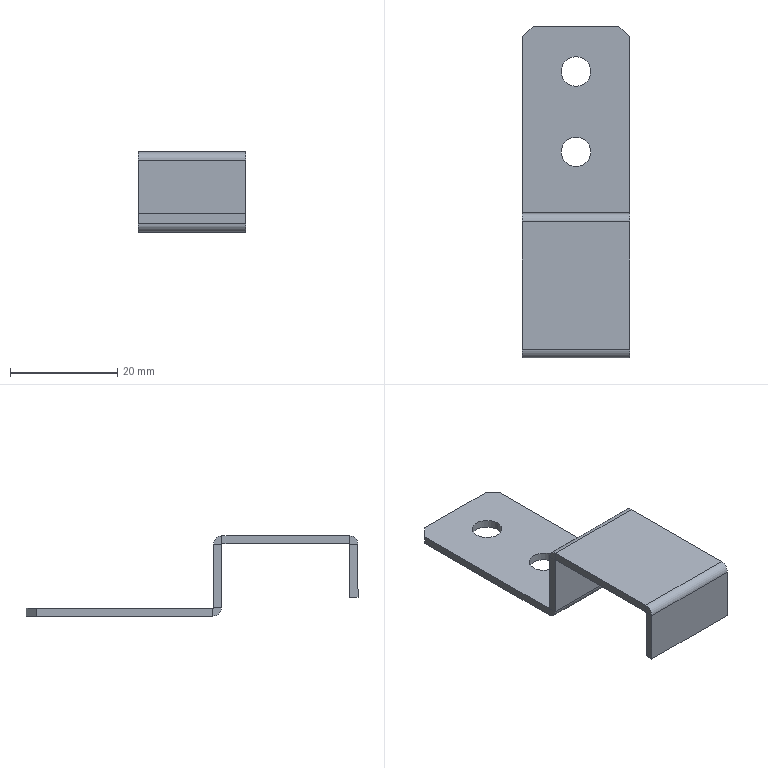Part | SolidWorks | features SplitBody 1 | 1 solid | 36 faces | box 20 x 62 x 15 mm | volume 2455 mm3 | plane 26 | cylinder 10 | commonest cylinder face diameters 5.5 x4 0.2 x3 3.2 x3
STEP:
#1=CARTESIAN_POINT('',(-247.25,40.,-280.));
#2=VERTEX_POINT('',#1);
#3=CARTESIAN_POINT('',(-252.75,40.,-280.));
#4=VERTEX_POINT('',#3);
#5=CARTESIAN_POINT('',(-250.,40.,-280.));
#6=DIRECTION('',(0.,0.,-1.));
#7=DIRECTION('',(-1.,0.,0.));
#8=AXIS2_PLACEMENT_3D('',#5,#6,#7);
#9=CIRCLE('',#8,2.75);
#10=EDGE_CURVE('',#2,#4,#9,.T.);
#11=ORIENTED_EDGE('',*,*,#10,.F.);
#12=CARTESIAN_POINT('',(-247.25,40.,-281.5));
#13=VERTEX_POINT('',#12);
#14=CARTESIAN_POINT('',(-247.25,40.,-221.5));
#15=DIRECTION('',(0.,0.,-1.));
#16=VECTOR('',#15,1000.);
#17=LINE('',#14,#16);
#18=EDGE_CURVE('',#2,#13,#17,.T.);
#19=ORIENTED_EDGE('',*,*,#18,.T.);
#20=CARTESIAN_POINT('',(-252.75,40.,-281.5));
#21=VERTEX_POINT('',#20);
#22=CARTESIAN_POINT('',(-250.,40.,-281.5));
#23=DIRECTION('',(0.,0.,-1.));
#24=DIRECTION('',(-1.,0.,0.));
#25=AXIS2_PLACEMENT_3D('',#22,#23,#24);
#26=CIRCLE('',#25,2.75);
#27=EDGE_CURVE('',#13,#21,#26,.T.);
#28=ORIENTED_EDGE('',*,*,#27,.T.);
#29=CARTESIAN_POINT('',(-252.75,40.,-221.5));
#30=DIRECTION('',(0.,0.,-1.));
#31=VECTOR('',#30,1000.);
#32=LINE('',#29,#31);
#33=EDGE_CURVE('',#4,#21,#32,.T.);
#34=ORIENTED_EDGE('',*,*,#33,.F.);
#35=EDGE_LOOP('',(#11,#19,#28,#34));
#36=FACE_OUTER_BOUND('',#35,.T.);
#37=CARTESIAN_POINT('',(-250.,40.,-221.5));
#38=DIRECTION('',(0.,0.,-1.));
#39=DIRECTION('',(-1.,0.,0.));
#40=AXIS2_PLACEMENT_3D('',#37,#38,#39);
#41=CYLINDRICAL_SURFACE('',#40,2.75);
#42=ADVANCED_FACE('',(#36),#41,.F.);
#43=CARTESIAN_POINT('',(-247.25,55.,-280.));
#44=VERTEX_POINT('',#43);
#45=CARTESIAN_POINT('',(-252.75,55.,-280.));
#46=VERTEX_POINT('',#45);
#47=CARTESIAN_POINT('',(-250.,55.,-280.));
#48=DIRECTION('',(0.,0.,-1.));
#49=DIRECTION('',(-1.,0.,0.));
#50=AXIS2_PLACEMENT_3D('',#47,#48,#49);
#51=CIRCLE('',#50,2.75);
#52=EDGE_CURVE('',#44,#46,#51,.T.);
#53=ORIENTED_EDGE('',*,*,#52,.F.);
#54=CARTESIAN_POINT('',(-247.25,55.,-281.5));
#55=VERTEX_POINT('',#54);
#56=CARTESIAN_POINT('',(-247.25,55.,-221.5));
#57=DIRECTION('',(0.,0.,-1.));
#58=VECTOR('',#57,1000.);
#59=LINE('',#56,#58);
#60=EDGE_CURVE('',#44,#55,#59,.T.);
#61=ORIENTED_EDGE('',*,*,#60,.T.);
#62=CARTESIAN_POINT('',(-252.75,55.,-281.5));
#63=VERTEX_POINT('',#62);
#64=CARTESIAN_POINT('',(-250.,55.,-281.5));
#65=DIRECTION('',(0.,0.,-1.));
#66=DIRECTION('',(-1.,0.,0.));
#67=AXIS2_PLACEMENT_3D('',#64,#65,#66);
#68=CIRCLE('',#67,2.75);
#69=EDGE_CURVE('',#55,#63,#68,.T.);
#70=ORIENTED_EDGE('',*,*,#69,.T.);
#71=CARTESIAN_POINT('',(-252.75,55.,-221.5));
#72=DIRECTION('',(0.,0.,-1.));
#73=VECTOR('',#72,1000.);
#74=LINE('',#71,#73);
#75=EDGE_CURVE('',#46,#63,#74,.T.);
#76=ORIENTED_EDGE('',*,*,#75,.F.);
#77=EDGE_LOOP('',(#53,#61,#70,#76));
#78=FACE_OUTER_BOUND('',#77,.T.);
#79=CARTESIAN_POINT('',(-250.,55.,-221.5));
#80=DIRECTION('',(0.,0.,-1.));
#81=DIRECTION('',(-1.,0.,0.));
#82=AXIS2_PLACEMENT_3D('',#79,#80,#81);
#83=CYLINDRICAL_SURFACE('',#82,2.75);
#84=ADVANCED_FACE('',(#78),#83,.F.);
#85=CARTESIAN_POINT('',(-260.,28.5,-279.9));
#86=VERTEX_POINT('',#85);
#87=CARTESIAN_POINT('',(-260.,27.,-279.9));
#88=VERTEX_POINT('',#87);
#89=CARTESIAN_POINT('',(-260.,28.5,-279.9));
#90=DIRECTION('',(0.,-1.,0.));
#91=VECTOR('',#90,1000.);
#92=LINE('',#89,#91);
#93=EDGE_CURVE('',#86,#88,#92,.T.);
#94=ORIENTED_EDGE('',*,*,#93,.T.);
#95=CARTESIAN_POINT('',(-260.,27.,-268.1));
#96=VERTEX_POINT('',#95);
#97=CARTESIAN_POINT('',(-260.,27.,-268.));
#98=DIRECTION('',(0.,0.,1.));
#99=VECTOR('',#98,1000.);
#100=LINE('',#97,#99);
#101=EDGE_CURVE('',#88,#96,#100,.T.);
#102=ORIENTED_EDGE('',*,*,#101,.T.);
#103=CARTESIAN_POINT('',(-260.,28.5,-268.1));
#104=VERTEX_POINT('',#103);
#105=CARTESIAN_POINT('',(-260.,28.5,-268.1));
#106=DIRECTION('',(0.,1.,0.));
#107=VECTOR('',#106,1000.);
#108=LINE('',#105,#107);
#109=EDGE_CURVE('',#96,#104,#108,.T.);
#110=ORIENTED_EDGE('',*,*,#109,.T.);
#111=CARTESIAN_POINT('',(-260.,28.5,0.));
#112=DIRECTION('',(0.,0.,1.));
#113=VECTOR('',#112,1000.);
#114=LINE('',#111,#113);
#115=EDGE_CURVE('',#86,#104,#114,.T.);
#116=ORIENTED_EDGE('',*,*,#115,.F.);
#117=EDGE_LOOP('',(#94,#102,#110,#116));
#118=FACE_OUTER_BOUND('',#117,.T.);
#119=CARTESIAN_POINT('',(-260.,28.5,-268.));
#120=DIRECTION('',(1.,0.,0.));
#121=DIRECTION('',(0.,1.,0.));
#122=AXIS2_PLACEMENT_3D('',#119,#120,#121);
#123=PLANE('',#122);
#124=ADVANCED_FACE('',(#118),#123,.F.);
#125=CARTESIAN_POINT('',(-240.,28.5,-279.9));
#126=VERTEX_POINT('',#125);
#127=CARTESIAN_POINT('',(-240.,27.,-279.9));
#128=VERTEX_POINT('',#127);
#129=CARTESIAN_POINT('',(-240.,28.5,-279.9));
#130=DIRECTION('',(0.,-1.,0.));
#131=VECTOR('',#130,1000.);
#132=LINE('',#129,#131);
#133=EDGE_CURVE('',#126,#128,#132,.T.);
#134=ORIENTED_EDGE('',*,*,#133,.F.);
#135=CARTESIAN_POINT('',(-240.,28.5,-268.1));
#136=VERTEX_POINT('',#135);
#137=CARTESIAN_POINT('',(-240.,28.5,0.));
#138=DIRECTION('',(0.,0.,-1.));
#139=VECTOR('',#138,1000.);
#140=LINE('',#137,#139);
#141=EDGE_CURVE('',#136,#126,#140,.T.);
#142=ORIENTED_EDGE('',*,*,#141,.F.);
#143=CARTESIAN_POINT('',(-240.,27.,-268.1));
#144=VERTEX_POINT('',#143);
#145=CARTESIAN_POINT('',(-240.,27.,-268.1));
#146=DIRECTION('',(0.,1.,0.));
#147=VECTOR('',#146,1000.);
#148=LINE('',#145,#147);
#149=EDGE_CURVE('',#144,#136,#148,.T.);
#150=ORIENTED_EDGE('',*,*,#149,.F.);
#151=CARTESIAN_POINT('',(-240.,27.,-280.));
#152=DIRECTION('',(0.,0.,-1.));
#153=VECTOR('',#152,1000.);
#154=LINE('',#151,#153);
#155=EDGE_CURVE('',#144,#128,#154,.T.);
#156=ORIENTED_EDGE('',*,*,#155,.T.);
#157=EDGE_LOOP('',(#134,#142,#150,#156));
#158=FACE_OUTER_BOUND('',#157,.T.);
#159=CARTESIAN_POINT('',(-240.,28.5,-280.));
#160=DIRECTION('',(-1.,0.,0.));
#161=DIRECTION('',(0.,-1.,0.));
#162=AXIS2_PLACEMENT_3D('',#159,#160,#161);
#163=PLANE('',#162);
#164=ADVANCED_FACE('',(#158),#163,.F.);
#165=CARTESIAN_POINT('',(-260.,28.5,-279.9));
#166=DIRECTION('',(1.,0.,0.));
#167=VECTOR('',#166,1000.);
#168=LINE('',#165,#167);
#169=EDGE_CURVE('',#86,#126,#168,.T.);
#170=ORIENTED_EDGE('',*,*,#169,.F.);
#171=ORIENTED_EDGE('',*,*,#115,.T.);
#172=CARTESIAN_POINT('',(-260.,28.5,-268.1));
#173=DIRECTION('',(-1.,0.,0.));
#174=VECTOR('',#173,1000.);
#175=LINE('',#172,#174);
#176=EDGE_CURVE('',#136,#104,#175,.T.);
#177=ORIENTED_EDGE('',*,*,#176,.F.);
#178=ORIENTED_EDGE('',*,*,#141,.T.);
#179=EDGE_LOOP('',(#170,#171,#177,#178));
#180=FACE_OUTER_BOUND('',#179,.T.);
#181=CARTESIAN_POINT('',(0.,28.5,0.));
#182=DIRECTION('',(0.,-1.,0.));
#183=DIRECTION('',(0.,0.,-1.));
#184=AXIS2_PLACEMENT_3D('',#181,#182,#183);
#185=PLANE('',#184);
#186=ADVANCED_FACE('',(#180),#185,.F.);
#187=ORIENTED_EDGE('',*,*,#101,.F.);
#188=CARTESIAN_POINT('',(-260.,27.,-279.9));
#189=DIRECTION('',(1.,0.,0.));
#190=VECTOR('',#189,1000.);
#191=LINE('',#188,#190);
#192=EDGE_CURVE('',#88,#128,#191,.T.);
#193=ORIENTED_EDGE('',*,*,#192,.T.);
#194=ORIENTED_EDGE('',*,*,#155,.F.);
#195=CARTESIAN_POINT('',(-260.,27.,-268.1));
#196=DIRECTION('',(1.,0.,0.));
#197=VECTOR('',#196,1000.);
#198=LINE('',#195,#197);
#199=EDGE_CURVE('',#96,#144,#198,.T.);
#200=ORIENTED_EDGE('',*,*,#199,.F.);
#201=EDGE_LOOP('',(#187,#193,#194,#200));
#202=FACE_OUTER_BOUND('',#201,.T.);
#203=CARTESIAN_POINT('',(0.,27.,0.));
#204=DIRECTION('',(0.,-1.,0.));
#205=DIRECTION('',(0.,0.,-1.));
#206=AXIS2_PLACEMENT_3D('',#203,#204,#205);
#207=PLANE('',#206);
#208=ADVANCED_FACE('',(#202),#207,.T.);
#209=CARTESIAN_POINT('',(-240.,3.1,-268.));
#210=VERTEX_POINT('',#209);
#211=CARTESIAN_POINT('',(-240.,3.1,-266.5));
#212=VERTEX_POINT('',#211);
#213=CARTESIAN_POINT('',(-240.,3.1,-268.));
#214=DIRECTION('',(0.,0.,1.));
#215=VECTOR('',#214,1000.);
#216=LINE('',#213,#215);
#217=EDGE_CURVE('',#210,#212,#216,.T.);
#218=ORIENTED_EDGE('',*,*,#217,.F.);
#219=CARTESIAN_POINT('',(-240.,26.9,-268.));
#220=VERTEX_POINT('',#219);
#221=CARTESIAN_POINT('',(-240.,28.5,-268.));
#222=DIRECTION('',(0.,-1.,0.));
#223=VECTOR('',#222,1000.);
#224=LINE('',#221,#223);
#225=EDGE_CURVE('',#220,#210,#224,.T.);
#226=ORIENTED_EDGE('',*,*,#225,.F.);
#227=CARTESIAN_POINT('',(-240.,26.9,-266.5));
#228=VERTEX_POINT('',#227);
#229=CARTESIAN_POINT('',(-240.,26.9,-268.));
#230=DIRECTION('',(0.,0.,1.));
#231=VECTOR('',#230,1000.);
#232=LINE('',#229,#231);
#233=EDGE_CURVE('',#220,#228,#232,.T.);
#234=ORIENTED_EDGE('',*,*,#233,.T.);
#235=CARTESIAN_POINT('',(-240.,28.5,-266.5));
#236=DIRECTION('',(0.,-1.,0.));
#237=VECTOR('',#236,1000.);
#238=LINE('',#235,#237);
#239=EDGE_CURVE('',#228,#212,#238,.T.);
#240=ORIENTED_EDGE('',*,*,#239,.T.);
#241=EDGE_LOOP('',(#218,#226,#234,#240));
#242=FACE_OUTER_BOUND('',#241,.T.);
#243=CARTESIAN_POINT('',(-240.,28.5,-268.));
#244=DIRECTION('',(-1.,0.,0.));
#245=DIRECTION('',(0.,0.,1.));
#246=AXIS2_PLACEMENT_3D('',#243,#244,#245);
#247=PLANE('',#246);
#248=ADVANCED_FACE('',(#242),#247,.F.);
#249=CARTESIAN_POINT('',(-260.,3.1,-268.));
#250=VERTEX_POINT('',#249);
#251=CARTESIAN_POINT('',(-260.,3.1,-266.5));
#252=VERTEX_POINT('',#251);
#253=CARTESIAN_POINT('',(-260.,3.1,-268.));
#254=DIRECTION('',(0.,0.,1.));
#255=VECTOR('',#254,1000.);
#256=LINE('',#253,#255);
#257=EDGE_CURVE('',#250,#252,#256,.T.);
#258=ORIENTED_EDGE('',*,*,#257,.T.);
#259=CARTESIAN_POINT('',(-260.,26.9,-266.5));
#260=VERTEX_POINT('',#259);
#261=CARTESIAN_POINT('',(-260.,28.5,-266.5));
#262=DIRECTION('',(0.,1.,0.));
#263=VECTOR('',#262,1000.);
#264=LINE('',#261,#263);
#265=EDGE_CURVE('',#252,#260,#264,.T.);
#266=ORIENTED_EDGE('',*,*,#265,.T.);
#267=CARTESIAN_POINT('',(-260.,26.9,-268.));
#268=VERTEX_POINT('',#267);
#269=CARTESIAN_POINT('',(-260.,26.9,-268.));
#270=DIRECTION('',(0.,0.,1.));
#271=VECTOR('',#270,1000.);
#272=LINE('',#269,#271);
#273=EDGE_CURVE('',#268,#260,#272,.T.);
#274=ORIENTED_EDGE('',*,*,#273,.F.);
#275=CARTESIAN_POINT('',(-260.,28.5,-268.));
#276=DIRECTION('',(0.,1.,0.));
#277=VECTOR('',#276,1000.);
#278=LINE('',#275,#277);
#279=EDGE_CURVE('',#250,#268,#278,.T.);
#280=ORIENTED_EDGE('',*,*,#279,.F.);
#281=EDGE_LOOP('',(#258,#266,#274,#280));
#282=FACE_OUTER_BOUND('',#281,.T.);
#283=CARTESIAN_POINT('',(-260.,28.5,-268.));
#284=DIRECTION('',(1.,0.,0.));
#285=DIRECTION('',(0.,0.,-1.));
#286=AXIS2_PLACEMENT_3D('',#283,#284,#285);
#287=PLANE('',#286);
#288=ADVANCED_FACE('',(#282),#287,.F.);
#289=ORIENTED_EDGE('',*,*,#225,.T.);
#290=CARTESIAN_POINT('',(-260.,3.1,-268.));
#291=DIRECTION('',(1.,0.,0.));
#292=VECTOR('',#291,1000.);
#293=LINE('',#290,#292);
#294=EDGE_CURVE('',#250,#210,#293,.T.);
#295=ORIENTED_EDGE('',*,*,#294,.F.);
#296=ORIENTED_EDGE('',*,*,#279,.T.);
#297=CARTESIAN_POINT('',(-240.,26.9,-268.));
#298=DIRECTION('',(-1.,0.,0.));
#299=VECTOR('',#298,1000.);
#300=LINE('',#297,#299);
#301=EDGE_CURVE('',#220,#268,#300,.T.);
#302=ORIENTED_EDGE('',*,*,#301,.F.);
#303=EDGE_LOOP('',(#289,#295,#296,#302));
#304=FACE_OUTER_BOUND('',#303,.T.);
#305=CARTESIAN_POINT('',(0.,0.,-268.));
#306=DIRECTION('',(0.,0.,-1.));
#307=DIRECTION('',(-1.,0.,0.));
#308=AXIS2_PLACEMENT_3D('',#305,#306,#307);
#309=PLANE('',#308);
#310=ADVANCED_FACE('',(#304),#309,.T.);
#311=CARTESIAN_POINT('',(-260.,3.1,-266.5));
#312=DIRECTION('',(1.,0.,0.));
#313=VECTOR('',#312,1000.);
#314=LINE('',#311,#313);
#315=EDGE_CURVE('',#252,#212,#314,.T.);
#316=ORIENTED_EDGE('',*,*,#315,.T.);
#317=ORIENTED_EDGE('',*,*,#239,.F.);
#318=CARTESIAN_POINT('',(-240.,26.9,-266.5));
#319=DIRECTION('',(-1.,0.,0.));
#320=VECTOR('',#319,1000.);
#321=LINE('',#318,#320);
#322=EDGE_CURVE('',#228,#260,#321,.T.);
#323=ORIENTED_EDGE('',*,*,#322,.T.);
#324=ORIENTED_EDGE('',*,*,#265,.F.);
#325=EDGE_LOOP('',(#316,#317,#323,#324));
#326=FACE_OUTER_BOUND('',#325,.T.);
#327=CARTESIAN_POINT('',(0.,0.,-266.5));
#328=DIRECTION('',(0.,0.,-1.));
#329=DIRECTION('',(-1.,0.,0.));
#330=AXIS2_PLACEMENT_3D('',#327,#328,#329);
#331=PLANE('',#330);
#332=ADVANCED_FACE('',(#326),#331,.F.);
#333=ORIENTED_EDGE('',*,*,#109,.F.);
#334=CARTESIAN_POINT('',(-260.,26.9,-268.1));
#335=DIRECTION('',(-1.,0.,0.));
#336=DIRECTION('',(0.,0.,-1.));
#337=AXIS2_PLACEMENT_3D('',#334,#335,#336);
#338=CIRCLE('',#337,0.1);
#339=EDGE_CURVE('',#268,#96,#338,.T.);
#340=ORIENTED_EDGE('',*,*,#339,.F.);
#341=ORIENTED_EDGE('',*,*,#273,.T.);
#342=CARTESIAN_POINT('',(-260.,26.9,-268.1));
#343=DIRECTION('',(-1.,0.,0.));
#344=DIRECTION('',(0.,0.,-1.));
#345=AXIS2_PLACEMENT_3D('',#342,#343,#344);
#346=CIRCLE('',#345,1.6);
#347=EDGE_CURVE('',#260,#104,#346,.T.);
#348=ORIENTED_EDGE('',*,*,#347,.T.);
#349=EDGE_LOOP('',(#333,#340,#341,#348));
#350=FACE_OUTER_BOUND('',#349,.T.);
#351=CARTESIAN_POINT('',(-260.,26.9,-268.1));
#352=DIRECTION('',(-1.,0.,0.));
#353=DIRECTION('',(0.,0.,1.));
#354=AXIS2_PLACEMENT_3D('',#351,#352,#353);
#355=PLANE('',#354);
#356=ADVANCED_FACE('',(#350),#355,.T.);
#357=CARTESIAN_POINT('',(-240.,26.9,-268.1));
#358=DIRECTION('',(1.,0.,0.));
#359=DIRECTION('',(0.,0.,-1.));
#360=AXIS2_PLACEMENT_3D('',#357,#358,#359);
#361=CIRCLE('',#360,0.1);
#362=EDGE_CURVE('',#144,#220,#361,.T.);
#363=ORIENTED_EDGE('',*,*,#362,.F.);
#364=ORIENTED_EDGE('',*,*,#149,.T.);
#365=CARTESIAN_POINT('',(-240.,26.9,-268.1));
#366=DIRECTION('',(1.,0.,0.));
#367=DIRECTION('',(0.,0.,-1.));
#368=AXIS2_PLACEMENT_3D('',#365,#366,#367);
#369=CIRCLE('',#368,1.6);
#370=EDGE_CURVE('',#136,#228,#369,.T.);
#371=ORIENTED_EDGE('',*,*,#370,.T.);
#372=ORIENTED_EDGE('',*,*,#233,.F.);
#373=EDGE_LOOP('',(#363,#364,#371,#372));
#374=FACE_OUTER_BOUND('',#373,.T.);
#375=CARTESIAN_POINT('',(-240.,26.9,-268.1));
#376=DIRECTION('',(-1.,0.,0.));
#377=DIRECTION('',(0.,0.,1.));
#378=AXIS2_PLACEMENT_3D('',#375,#376,#377);
#379=PLANE('',#378);
#380=ADVANCED_FACE('',(#374),#379,.F.);
#381=ORIENTED_EDGE('',*,*,#322,.F.);
#382=ORIENTED_EDGE('',*,*,#370,.F.);
#383=ORIENTED_EDGE('',*,*,#176,.T.);
#384=ORIENTED_EDGE('',*,*,#347,.F.);
#385=EDGE_LOOP('',(#381,#382,#383,#384));
#386=FACE_OUTER_BOUND('',#385,.T.);
#387=CARTESIAN_POINT('',(-240.,26.9,-268.1));
#388=DIRECTION('',(1.,0.,0.));
#389=DIRECTION('',(0.,1.,0.));
#390=AXIS2_PLACEMENT_3D('',#387,#388,#389);
#391=CYLINDRICAL_SURFACE('',#390,1.6);
#392=ADVANCED_FACE('',(#386),#391,.T.);
#393=ORIENTED_EDGE('',*,*,#301,.T.);
#394=ORIENTED_EDGE('',*,*,#339,.T.);
#395=ORIENTED_EDGE('',*,*,#199,.T.);
#396=ORIENTED_EDGE('',*,*,#362,.T.);
#397=EDGE_LOOP('',(#393,#394,#395,#396));
#398=FACE_OUTER_BOUND('',#397,.T.);
#399=CARTESIAN_POINT('',(-240.,26.9,-268.1));
#400=DIRECTION('',(1.,0.,0.));
#401=DIRECTION('',(0.,1.,0.));
#402=AXIS2_PLACEMENT_3D('',#399,#400,#401);
#403=CYLINDRICAL_SURFACE('',#402,0.1);
#404=ADVANCED_FACE('',(#398),#403,.F.);
#405=CARTESIAN_POINT('',(-240.,3.,-268.1));
#406=VERTEX_POINT('',#405);
#407=CARTESIAN_POINT('',(-240.,1.5,-268.1));
#408=VERTEX_POINT('',#407);
#409=CARTESIAN_POINT('',(-240.,1.5,-268.1));
#410=DIRECTION('',(0.,-1.,0.));
#411=VECTOR('',#410,1000.);
#412=LINE('',#409,#411);
#413=EDGE_CURVE('',#406,#408,#412,.T.);
#414=ORIENTED_EDGE('',*,*,#413,.F.);
#415=CARTESIAN_POINT('',(-240.,3.1,-268.1));
#416=DIRECTION('',(1.,0.,0.));
#417=DIRECTION('',(0.,0.,1.));
#418=AXIS2_PLACEMENT_3D('',#415,#416,#417);
#419=CIRCLE('',#418,0.1);
#420=EDGE_CURVE('',#210,#406,#419,.T.);
#421=ORIENTED_EDGE('',*,*,#420,.F.);
#422=ORIENTED_EDGE('',*,*,#217,.T.);
#423=CARTESIAN_POINT('',(-240.,3.1,-268.1));
#424=DIRECTION('',(1.,0.,0.));
#425=DIRECTION('',(0.,0.,1.));
#426=AXIS2_PLACEMENT_3D('',#423,#424,#425);
#427=CIRCLE('',#426,1.6);
#428=EDGE_CURVE('',#212,#408,#427,.T.);
#429=ORIENTED_EDGE('',*,*,#428,.T.);
#430=EDGE_LOOP('',(#414,#421,#422,#429));
#431=FACE_OUTER_BOUND('',#430,.T.);
#432=CARTESIAN_POINT('',(-240.,3.1,-268.1));
#433=DIRECTION('',(1.,0.,0.));
#434=DIRECTION('',(0.,0.,-1.));
#435=AXIS2_PLACEMENT_3D('',#432,#433,#434);
#436=PLANE('',#435);
#437=ADVANCED_FACE('',(#431),#436,.T.);
#438=CARTESIAN_POINT('',(-260.,3.,-268.1));
#439=VERTEX_POINT('',#438);
#440=CARTESIAN_POINT('',(-260.,3.1,-268.1));
#441=DIRECTION('',(-1.,0.,0.));
#442=DIRECTION('',(0.,0.,1.));
#443=AXIS2_PLACEMENT_3D('',#440,#441,#442);
#444=CIRCLE('',#443,0.1);
#445=EDGE_CURVE('',#439,#250,#444,.T.);
#446=ORIENTED_EDGE('',*,*,#445,.F.);
#447=CARTESIAN_POINT('',(-260.,1.5,-268.1));
#448=VERTEX_POINT('',#447);
#449=CARTESIAN_POINT('',(-260.,3.,-268.1));
#450=DIRECTION('',(0.,-1.,0.));
#451=VECTOR('',#450,1000.);
#452=LINE('',#449,#451);
#453=EDGE_CURVE('',#439,#448,#452,.T.);
#454=ORIENTED_EDGE('',*,*,#453,.T.);
#455=CARTESIAN_POINT('',(-260.,3.1,-268.1));
#456=DIRECTION('',(-1.,0.,0.));
#457=DIRECTION('',(0.,0.,1.));
#458=AXIS2_PLACEMENT_3D('',#455,#456,#457);
#459=CIRCLE('',#458,1.6);
#460=EDGE_CURVE('',#448,#252,#459,.T.);
#461=ORIENTED_EDGE('',*,*,#460,.T.);
#462=ORIENTED_EDGE('',*,*,#257,.F.);
#463=EDGE_LOOP('',(#446,#454,#461,#462));
#464=FACE_OUTER_BOUND('',#463,.T.);
#465=CARTESIAN_POINT('',(-260.,3.1,-268.1));
#466=DIRECTION('',(1.,0.,0.));
#467=DIRECTION('',(0.,0.,-1.));
#468=AXIS2_PLACEMENT_3D('',#465,#466,#467);
#469=PLANE('',#468);
#470=ADVANCED_FACE('',(#464),#469,.F.);
#471=ORIENTED_EDGE('',*,*,#315,.F.);
#472=ORIENTED_EDGE('',*,*,#460,.F.);
#473=CARTESIAN_POINT('',(-240.,1.5,-268.1));
#474=DIRECTION('',(1.,0.,0.));
#475=VECTOR('',#474,1000.);
#476=LINE('',#473,#475);
#477=EDGE_CURVE('',#448,#408,#476,.T.);
#478=ORIENTED_EDGE('',*,*,#477,.T.);
#479=ORIENTED_EDGE('',*,*,#428,.F.);
#480=EDGE_LOOP('',(#471,#472,#478,#479));
#481=FACE_OUTER_BOUND('',#480,.T.);
#482=CARTESIAN_POINT('',(-260.,3.1,-268.1));
#483=DIRECTION('',(-1.,0.,0.));
#484=DIRECTION('',(0.,-1.,0.));
#485=AXIS2_PLACEMENT_3D('',#482,#483,#484);
#486=CYLINDRICAL_SURFACE('',#485,1.6);
#487=ADVANCED_FACE('',(#481),#486,.T.);
#488=ORIENTED_EDGE('',*,*,#294,.T.);
#489=ORIENTED_EDGE('',*,*,#420,.T.);
#490=CARTESIAN_POINT('',(-240.,3.,-268.1));
#491=DIRECTION('',(-1.,0.,0.));
#492=VECTOR('',#491,1000.);
#493=LINE('',#490,#492);
#494=EDGE_CURVE('',#406,#439,#493,.T.);
#495=ORIENTED_EDGE('',*,*,#494,.T.);
#496=ORIENTED_EDGE('',*,*,#445,.T.);
#497=EDGE_LOOP('',(#488,#489,#495,#496));
#498=FACE_OUTER_BOUND('',#497,.T.);
#499=CARTESIAN_POINT('',(-260.,3.1,-268.1));
#500=DIRECTION('',(-1.,0.,0.));
#501=DIRECTION('',(0.,-1.,0.));
#502=AXIS2_PLACEMENT_3D('',#499,#500,#501);
#503=CYLINDRICAL_SURFACE('',#502,0.1);
#504=ADVANCED_FACE('',(#498),#503,.F.);
#505=ORIENTED_EDGE('',*,*,#453,.F.);
#506=CARTESIAN_POINT('',(-260.,3.,-278.));
#507=VERTEX_POINT('',#506);
#508=CARTESIAN_POINT('',(-260.,3.,-278.));
#509=DIRECTION('',(0.,0.,-1.));
#510=VECTOR('',#509,1000.);
#511=LINE('',#508,#510);
#512=EDGE_CURVE('',#439,#507,#511,.T.);
#513=ORIENTED_EDGE('',*,*,#512,.T.);
#514=CARTESIAN_POINT('',(-260.,1.5,-278.));
#515=VERTEX_POINT('',#514);
#516=CARTESIAN_POINT('',(-260.,1.5,-278.));
#517=DIRECTION('',(0.,1.,0.));
#518=VECTOR('',#517,1000.);
#519=LINE('',#516,#518);
#520=EDGE_CURVE('',#515,#507,#519,.T.);
#521=ORIENTED_EDGE('',*,*,#520,.F.);
#522=CARTESIAN_POINT('',(-260.,1.5,0.));
#523=DIRECTION('',(0.,0.,-1.));
#524=VECTOR('',#523,1000.);
#525=LINE('',#522,#524);
#526=EDGE_CURVE('',#448,#515,#525,.T.);
#527=ORIENTED_EDGE('',*,*,#526,.F.);
#528=EDGE_LOOP('',(#505,#513,#521,#527));
#529=FACE_OUTER_BOUND('',#528,.T.);
#530=CARTESIAN_POINT('',(-260.,1.5,-278.));
#531=DIRECTION('',(1.,0.,0.));
#532=DIRECTION('',(0.,1.,0.));
#533=AXIS2_PLACEMENT_3D('',#530,#531,#532);
#534=PLANE('',#533);
#535=ADVANCED_FACE('',(#529),#534,.F.);
#536=ORIENTED_EDGE('',*,*,#413,.T.);
#537=CARTESIAN_POINT('',(-240.,1.5,-278.));
#538=VERTEX_POINT('',#537);
#539=CARTESIAN_POINT('',(-240.,1.5,0.));
#540=DIRECTION('',(0.,0.,1.));
#541=VECTOR('',#540,1000.);
#542=LINE('',#539,#541);
#543=EDGE_CURVE('',#538,#408,#542,.T.);
#544=ORIENTED_EDGE('',*,*,#543,.F.);
#545=CARTESIAN_POINT('',(-240.,3.,-278.));
#546=VERTEX_POINT('',#545);
#547=CARTESIAN_POINT('',(-240.,1.5,-278.));
#548=DIRECTION('',(0.,1.,0.));
#549=VECTOR('',#548,1000.);
#550=LINE('',#547,#549);
#551=EDGE_CURVE('',#538,#546,#550,.T.);
#552=ORIENTED_EDGE('',*,*,#551,.T.);
#553=CARTESIAN_POINT('',(-240.,3.,-268.));
#554=DIRECTION('',(0.,0.,1.));
#555=VECTOR('',#554,1000.);
#556=LINE('',#553,#555);
#557=EDGE_CURVE('',#546,#406,#556,.T.);
#558=ORIENTED_EDGE('',*,*,#557,.T.);
#559=EDGE_LOOP('',(#536,#544,#552,#558));
#560=FACE_OUTER_BOUND('',#559,.T.);
#561=CARTESIAN_POINT('',(-240.,1.5,-268.));
#562=DIRECTION('',(-1.,0.,0.));
#563=DIRECTION('',(0.,-1.,0.));
#564=AXIS2_PLACEMENT_3D('',#561,#562,#563);
#565=PLANE('',#564);
#566=ADVANCED_FACE('',(#560),#565,.F.);
#567=ORIENTED_EDGE('',*,*,#477,.F.);
#568=ORIENTED_EDGE('',*,*,#526,.T.);
#569=CARTESIAN_POINT('',(0.,1.5,-278.));
#570=DIRECTION('',(1.,0.,0.));
#571=VECTOR('',#570,1000.);
#572=LINE('',#569,#571);
#573=EDGE_CURVE('',#515,#538,#572,.T.);
#574=ORIENTED_EDGE('',*,*,#573,.T.);
#575=ORIENTED_EDGE('',*,*,#543,.T.);
#576=EDGE_LOOP('',(#567,#568,#574,#575));
#577=FACE_OUTER_BOUND('',#576,.T.);
#578=CARTESIAN_POINT('',(0.,1.5,0.));
#579=DIRECTION('',(0.,1.,0.));
#580=DIRECTION('',(0.,0.,1.));
#581=AXIS2_PLACEMENT_3D('',#578,#579,#580);
#582=PLANE('',#581);
#583=ADVANCED_FACE('',(#577),#582,.F.);
#584=ORIENTED_EDGE('',*,*,#512,.F.);
#585=ORIENTED_EDGE('',*,*,#494,.F.);
#586=ORIENTED_EDGE('',*,*,#557,.F.);
#587=CARTESIAN_POINT('',(-240.,3.,-278.));
#588=DIRECTION('',(1.,0.,0.));
#589=VECTOR('',#588,1000.);
#590=LINE('',#587,#589);
#591=EDGE_CURVE('',#507,#546,#590,.T.);
#592=ORIENTED_EDGE('',*,*,#591,.F.);
#593=EDGE_LOOP('',(#584,#585,#586,#592));
#594=FACE_OUTER_BOUND('',#593,.T.);
#595=CARTESIAN_POINT('',(0.,3.,0.));
#596=DIRECTION('',(0.,1.,0.));
#597=DIRECTION('',(0.,0.,1.));
#598=AXIS2_PLACEMENT_3D('',#595,#596,#597);
#599=PLANE('',#598);
#600=ADVANCED_FACE('',(#594),#599,.T.);
#601=ORIENTED_EDGE('',*,*,#591,.T.);
#602=ORIENTED_EDGE('',*,*,#551,.F.);
#603=ORIENTED_EDGE('',*,*,#573,.F.);
#604=ORIENTED_EDGE('',*,*,#520,.T.);
#605=EDGE_LOOP('',(#601,#602,#603,#604));
#606=FACE_OUTER_BOUND('',#605,.T.);
#607=CARTESIAN_POINT('',(-240.,1.5,-278.));
#608=DIRECTION('',(0.,0.,1.));
#609=DIRECTION('',(0.,-1.,0.));
#610=AXIS2_PLACEMENT_3D('',#607,#608,#609);
#611=PLANE('',#610);
#612=ADVANCED_FACE('',(#606),#611,.F.);
#613=CARTESIAN_POINT('',(-240.,28.6,-280.));
#614=VERTEX_POINT('',#613);
#615=CARTESIAN_POINT('',(-240.,28.6,-281.5));
#616=VERTEX_POINT('',#615);
#617=CARTESIAN_POINT('',(-240.,28.6,-280.));
#618=DIRECTION('',(0.,0.,-1.));
#619=VECTOR('',#618,1000.);
#620=LINE('',#617,#619);
#621=EDGE_CURVE('',#614,#616,#620,.T.);
#622=ORIENTED_EDGE('',*,*,#621,.F.);
#623=CARTESIAN_POINT('',(-240.,28.6,-279.9));
#624=DIRECTION('',(1.,0.,0.));
#625=DIRECTION('',(0.,0.,1.));
#626=AXIS2_PLACEMENT_3D('',#623,#624,#625);
#627=CIRCLE('',#626,0.1);
#628=EDGE_CURVE('',#126,#614,#627,.T.);
#629=ORIENTED_EDGE('',*,*,#628,.F.);
#630=ORIENTED_EDGE('',*,*,#133,.T.);
#631=CARTESIAN_POINT('',(-240.,28.6,-279.9));
#632=DIRECTION('',(1.,0.,0.));
#633=DIRECTION('',(0.,0.,1.));
#634=AXIS2_PLACEMENT_3D('',#631,#632,#633);
#635=CIRCLE('',#634,1.6);
#636=EDGE_CURVE('',#128,#616,#635,.T.);
#637=ORIENTED_EDGE('',*,*,#636,.T.);
#638=EDGE_LOOP('',(#622,#629,#630,#637));
#639=FACE_OUTER_BOUND('',#638,.T.);
#640=CARTESIAN_POINT('',(-240.,28.6,-279.9));
#641=DIRECTION('',(1.,0.,0.));
#642=DIRECTION('',(0.,0.,-1.));
#643=AXIS2_PLACEMENT_3D('',#640,#641,#642);
#644=PLANE('',#643);
#645=ADVANCED_FACE('',(#639),#644,.T.);
#646=CARTESIAN_POINT('',(-260.,28.6,-280.));
#647=VERTEX_POINT('',#646);
#648=CARTESIAN_POINT('',(-260.,28.6,-279.9));
#649=DIRECTION('',(-1.,0.,0.));
#650=DIRECTION('',(0.,0.,1.));
#651=AXIS2_PLACEMENT_3D('',#648,#649,#650);
#652=CIRCLE('',#651,0.1);
#653=EDGE_CURVE('',#647,#86,#652,.T.);
#654=ORIENTED_EDGE('',*,*,#653,.F.);
#655=CARTESIAN_POINT('',(-260.,28.6,-281.5));
#656=VERTEX_POINT('',#655);
#657=CARTESIAN_POINT('',(-260.,28.6,-280.));
#658=DIRECTION('',(0.,0.,-1.));
#659=VECTOR('',#658,1000.);
#660=LINE('',#657,#659);
#661=EDGE_CURVE('',#647,#656,#660,.T.);
#662=ORIENTED_EDGE('',*,*,#661,.T.);
#663=CARTESIAN_POINT('',(-260.,28.6,-279.9));
#664=DIRECTION('',(-1.,0.,0.));
#665=DIRECTION('',(0.,0.,1.));
#666=AXIS2_PLACEMENT_3D('',#663,#664,#665);
#667=CIRCLE('',#666,1.6);
#668=EDGE_CURVE('',#656,#88,#667,.T.);
#669=ORIENTED_EDGE('',*,*,#668,.T.);
#670=ORIENTED_EDGE('',*,*,#93,.F.);
#671=EDGE_LOOP('',(#654,#662,#669,#670));
#672=FACE_OUTER_BOUND('',#671,.T.);
#673=CARTESIAN_POINT('',(-260.,28.6,-279.9));
#674=DIRECTION('',(1.,0.,0.));
#675=DIRECTION('',(0.,0.,-1.));
#676=AXIS2_PLACEMENT_3D('',#673,#674,#675);
#677=PLANE('',#676);
#678=ADVANCED_FACE('',(#672),#677,.F.);
#679=ORIENTED_EDGE('',*,*,#192,.F.);
#680=ORIENTED_EDGE('',*,*,#668,.F.);
#681=CARTESIAN_POINT('',(0.,28.6,-281.5));
#682=DIRECTION('',(-1.,0.,0.));
#683=VECTOR('',#682,1000.);
#684=LINE('',#681,#683);
#685=EDGE_CURVE('',#616,#656,#684,.T.);
#686=ORIENTED_EDGE('',*,*,#685,.F.);
#687=ORIENTED_EDGE('',*,*,#636,.F.);
#688=EDGE_LOOP('',(#679,#680,#686,#687));
#689=FACE_OUTER_BOUND('',#688,.T.);
#690=CARTESIAN_POINT('',(-260.,28.6,-279.9));
#691=DIRECTION('',(-1.,0.,0.));
#692=DIRECTION('',(0.,0.,-1.));
#693=AXIS2_PLACEMENT_3D('',#690,#691,#692);
#694=CYLINDRICAL_SURFACE('',#693,1.6);
#695=ADVANCED_FACE('',(#689),#694,.T.);
#696=ORIENTED_EDGE('',*,*,#169,.T.);
#697=ORIENTED_EDGE('',*,*,#628,.T.);
#698=CARTESIAN_POINT('',(-240.,28.6,-280.));
#699=DIRECTION('',(-1.,0.,0.));
#700=VECTOR('',#699,1000.);
#701=LINE('',#698,#700);
#702=EDGE_CURVE('',#614,#647,#701,.T.);
#703=ORIENTED_EDGE('',*,*,#702,.T.);
#704=ORIENTED_EDGE('',*,*,#653,.T.);
#705=EDGE_LOOP('',(#696,#697,#703,#704));
#706=FACE_OUTER_BOUND('',#705,.T.);
#707=CARTESIAN_POINT('',(-260.,28.6,-279.9));
#708=DIRECTION('',(-1.,0.,0.));
#709=DIRECTION('',(0.,0.,-1.));
#710=AXIS2_PLACEMENT_3D('',#707,#708,#709);
#711=CYLINDRICAL_SURFACE('',#710,0.1);
#712=ADVANCED_FACE('',(#706),#711,.F.);
#713=CARTESIAN_POINT('',(-260.,61.5,-280.));
#714=VERTEX_POINT('',#713);
#715=CARTESIAN_POINT('',(-260.,28.5,-280.));
#716=DIRECTION('',(0.,-1.,0.));
#717=VECTOR('',#716,1000.);
#718=LINE('',#715,#717);
#719=EDGE_CURVE('',#714,#647,#718,.T.);
#720=ORIENTED_EDGE('',*,*,#719,.F.);
#721=CARTESIAN_POINT('',(-260.,61.5,-281.5));
#722=VERTEX_POINT('',#721);
#723=CARTESIAN_POINT('',(-260.,61.5,-281.5));
#724=DIRECTION('',(0.,0.,-1.));
#725=VECTOR('',#724,1000.);
#726=LINE('',#723,#725);
#727=EDGE_CURVE('',#714,#722,#726,.T.);
#728=ORIENTED_EDGE('',*,*,#727,.T.);
#729=CARTESIAN_POINT('',(-260.,28.5,-281.5));
#730=DIRECTION('',(0.,-1.,0.));
#731=VECTOR('',#730,1000.);
#732=LINE('',#729,#731);
#733=EDGE_CURVE('',#722,#656,#732,.T.);
#734=ORIENTED_EDGE('',*,*,#733,.T.);
#735=ORIENTED_EDGE('',*,*,#661,.F.);
#736=EDGE_LOOP('',(#720,#728,#734,#735));
#737=FACE_OUTER_BOUND('',#736,.T.);
#738=CARTESIAN_POINT('',(-260.,28.5,-281.5));
#739=DIRECTION('',(-1.,0.,0.));
#740=DIRECTION('',(0.,0.,1.));
#741=AXIS2_PLACEMENT_3D('',#738,#739,#740);
#742=PLANE('',#741);
#743=ADVANCED_FACE('',(#737),#742,.T.);
#744=CARTESIAN_POINT('',(-240.,61.5,-281.5));
#745=VERTEX_POINT('',#744);
#746=CARTESIAN_POINT('',(-240.,63.5,-281.5));
#747=DIRECTION('',(0.,1.,0.));
#748=VECTOR('',#747,1000.);
#749=LINE('',#746,#748);
#750=EDGE_CURVE('',#616,#745,#749,.T.);
#751=ORIENTED_EDGE('',*,*,#750,.T.);
#752=CARTESIAN_POINT('',(-240.,61.5,-280.));
#753=VERTEX_POINT('',#752);
#754=CARTESIAN_POINT('',(-240.,61.5,-281.5));
#755=DIRECTION('',(0.,0.,1.));
#756=VECTOR('',#755,1000.);
#757=LINE('',#754,#756);
#758=EDGE_CURVE('',#745,#753,#757,.T.);
#759=ORIENTED_EDGE('',*,*,#758,.T.);
#760=CARTESIAN_POINT('',(-240.,63.5,-280.));
#761=DIRECTION('',(0.,1.,0.));
#762=VECTOR('',#761,1000.);
#763=LINE('',#760,#762);
#764=EDGE_CURVE('',#614,#753,#763,.T.);
#765=ORIENTED_EDGE('',*,*,#764,.F.);
#766=ORIENTED_EDGE('',*,*,#621,.T.);
#767=EDGE_LOOP('',(#751,#759,#765,#766));
#768=FACE_OUTER_BOUND('',#767,.T.);
#769=CARTESIAN_POINT('',(-240.,63.5,-281.5));
#770=DIRECTION('',(1.,0.,0.));
#771=DIRECTION('',(0.,0.,-1.));
#772=AXIS2_PLACEMENT_3D('',#769,#770,#771);
#773=PLANE('',#772);
#774=ADVANCED_FACE('',(#768),#773,.T.);
#775=CARTESIAN_POINT('',(-250.,40.,-281.5));
#776=DIRECTION('',(0.,0.,-1.));
#777=DIRECTION('',(-1.,0.,0.));
#778=AXIS2_PLACEMENT_3D('',#775,#776,#777);
#779=CIRCLE('',#778,2.75);
#780=EDGE_CURVE('',#21,#13,#779,.T.);
#781=ORIENTED_EDGE('',*,*,#780,.F.);
#782=ORIENTED_EDGE('',*,*,#27,.F.);
#783=EDGE_LOOP('',(#781,#782));
#784=FACE_BOUND('',#783,.T.);
#785=CARTESIAN_POINT('',(-250.,55.,-281.5));
#786=DIRECTION('',(0.,0.,-1.));
#787=DIRECTION('',(-1.,0.,0.));
#788=AXIS2_PLACEMENT_3D('',#785,#786,#787);
#789=CIRCLE('',#788,2.75);
#790=EDGE_CURVE('',#63,#55,#789,.T.);
#791=ORIENTED_EDGE('',*,*,#790,.F.);
#792=ORIENTED_EDGE('',*,*,#69,.F.);
#793=EDGE_LOOP('',(#791,#792));
#794=FACE_BOUND('',#793,.T.);
#795=ORIENTED_EDGE('',*,*,#733,.F.);
#796=CARTESIAN_POINT('',(-258.,63.5,-281.5));
#797=VERTEX_POINT('',#796);
#798=CARTESIAN_POINT('',(-160.75,160.75,-281.5));
#799=DIRECTION('',(0.7071,0.7071,0.));
#800=VECTOR('',#799,1000.);
#801=LINE('',#798,#800);
#802=EDGE_CURVE('',#722,#797,#801,.T.);
#803=ORIENTED_EDGE('',*,*,#802,.T.);
#804=CARTESIAN_POINT('',(-242.,63.5,-281.5));
#805=VERTEX_POINT('',#804);
#806=CARTESIAN_POINT('',(-260.,63.5,-281.5));
#807=DIRECTION('',(-1.,0.,0.));
#808=VECTOR('',#807,1000.);
#809=LINE('',#806,#808);
#810=EDGE_CURVE('',#805,#797,#809,.T.);
#811=ORIENTED_EDGE('',*,*,#810,.F.);
#812=CARTESIAN_POINT('',(-89.25,-89.25,-281.5));
#813=DIRECTION('',(0.7071,-0.7071,0.));
#814=VECTOR('',#813,1000.);
#815=LINE('',#812,#814);
#816=EDGE_CURVE('',#805,#745,#815,.T.);
#817=ORIENTED_EDGE('',*,*,#816,.T.);
#818=ORIENTED_EDGE('',*,*,#750,.F.);
#819=ORIENTED_EDGE('',*,*,#685,.T.);
#820=EDGE_LOOP('',(#795,#803,#811,#817,#818,#819));
#821=FACE_OUTER_BOUND('',#820,.T.);
#822=CARTESIAN_POINT('',(0.,0.,-281.5));
#823=DIRECTION('',(0.,0.,-1.));
#824=DIRECTION('',(-1.,0.,0.));
#825=AXIS2_PLACEMENT_3D('',#822,#823,#824);
#826=PLANE('',#825);
#827=ADVANCED_FACE('',(#784,#794,#821),#826,.T.);
#828=CARTESIAN_POINT('',(-250.,40.,-280.));
#829=DIRECTION('',(0.,0.,-1.));
#830=DIRECTION('',(-1.,0.,0.));
#831=AXIS2_PLACEMENT_3D('',#828,#829,#830);
#832=CIRCLE('',#831,2.75);
#833=EDGE_CURVE('',#4,#2,#832,.T.);
#834=ORIENTED_EDGE('',*,*,#833,.T.);
#835=ORIENTED_EDGE('',*,*,#10,.T.);
#836=EDGE_LOOP('',(#834,#835));
#837=FACE_BOUND('',#836,.T.);
#838=CARTESIAN_POINT('',(-250.,55.,-280.));
#839=DIRECTION('',(0.,0.,-1.));
#840=DIRECTION('',(-1.,0.,0.));
#841=AXIS2_PLACEMENT_3D('',#838,#839,#840);
#842=CIRCLE('',#841,2.75);
#843=EDGE_CURVE('',#46,#44,#842,.T.);
#844=ORIENTED_EDGE('',*,*,#843,.T.);
#845=ORIENTED_EDGE('',*,*,#52,.T.);
#846=EDGE_LOOP('',(#844,#845));
#847=FACE_BOUND('',#846,.T.);
#848=CARTESIAN_POINT('',(-242.,63.5,-280.));
#849=VERTEX_POINT('',#848);
#850=CARTESIAN_POINT('',(-258.,63.5,-280.));
#851=VERTEX_POINT('',#850);
#852=CARTESIAN_POINT('',(-260.,63.5,-280.));
#853=DIRECTION('',(-1.,0.,0.));
#854=VECTOR('',#853,1000.);
#855=LINE('',#852,#854);
#856=EDGE_CURVE('',#849,#851,#855,.T.);
#857=ORIENTED_EDGE('',*,*,#856,.T.);
#858=CARTESIAN_POINT('',(-258.,63.5,-280.));
#859=DIRECTION('',(-0.7071,-0.7071,0.));
#860=VECTOR('',#859,1000.);
#861=LINE('',#858,#860);
#862=EDGE_CURVE('',#851,#714,#861,.T.);
#863=ORIENTED_EDGE('',*,*,#862,.T.);
#864=ORIENTED_EDGE('',*,*,#719,.T.);
#865=ORIENTED_EDGE('',*,*,#702,.F.);
#866=ORIENTED_EDGE('',*,*,#764,.T.);
#867=CARTESIAN_POINT('',(-240.,61.5,-280.));
#868=DIRECTION('',(-0.7071,0.7071,0.));
#869=VECTOR('',#868,1000.);
#870=LINE('',#867,#869);
#871=EDGE_CURVE('',#753,#849,#870,.T.);
#872=ORIENTED_EDGE('',*,*,#871,.T.);
#873=EDGE_LOOP('',(#857,#863,#864,#865,#866,#872));
#874=FACE_OUTER_BOUND('',#873,.T.);
#875=CARTESIAN_POINT('',(0.,0.,-280.));
#876=DIRECTION('',(0.,0.,-1.));
#877=DIRECTION('',(-1.,0.,0.));
#878=AXIS2_PLACEMENT_3D('',#875,#876,#877);
#879=PLANE('',#878);
#880=ADVANCED_FACE('',(#837,#847,#874),#879,.F.);
#881=ORIENTED_EDGE('',*,*,#810,.T.);
#882=CARTESIAN_POINT('',(-258.,63.5,-281.5));
#883=DIRECTION('',(0.,0.,1.));
#884=VECTOR('',#883,1000.);
#885=LINE('',#882,#884);
#886=EDGE_CURVE('',#797,#851,#885,.T.);
#887=ORIENTED_EDGE('',*,*,#886,.T.);
#888=ORIENTED_EDGE('',*,*,#856,.F.);
#889=CARTESIAN_POINT('',(-242.,63.5,-281.5));
#890=DIRECTION('',(0.,0.,-1.));
#891=VECTOR('',#890,1000.);
#892=LINE('',#889,#891);
#893=EDGE_CURVE('',#849,#805,#892,.T.);
#894=ORIENTED_EDGE('',*,*,#893,.T.);
#895=EDGE_LOOP('',(#881,#887,#888,#894));
#896=FACE_OUTER_BOUND('',#895,.T.);
#897=CARTESIAN_POINT('',(-260.,63.5,-281.5));
#898=DIRECTION('',(0.,1.,0.));
#899=DIRECTION('',(0.,0.,1.));
#900=AXIS2_PLACEMENT_3D('',#897,#898,#899);
#901=PLANE('',#900);
#902=ADVANCED_FACE('',(#896),#901,.T.);
#903=ORIENTED_EDGE('',*,*,#60,.F.);
#904=ORIENTED_EDGE('',*,*,#843,.F.);
#905=ORIENTED_EDGE('',*,*,#75,.T.);
#906=ORIENTED_EDGE('',*,*,#790,.T.);
#907=EDGE_LOOP('',(#903,#904,#905,#906));
#908=FACE_OUTER_BOUND('',#907,.T.);
#909=CARTESIAN_POINT('',(-250.,55.,-221.5));
#910=DIRECTION('',(0.,0.,-1.));
#911=DIRECTION('',(-1.,0.,0.));
#912=AXIS2_PLACEMENT_3D('',#909,#910,#911);
#913=CYLINDRICAL_SURFACE('',#912,2.75);
#914=ADVANCED_FACE('',(#908),#913,.F.);
#915=ORIENTED_EDGE('',*,*,#18,.F.);
#916=ORIENTED_EDGE('',*,*,#833,.F.);
#917=ORIENTED_EDGE('',*,*,#33,.T.);
#918=ORIENTED_EDGE('',*,*,#780,.T.);
#919=EDGE_LOOP('',(#915,#916,#917,#918));
#920=FACE_OUTER_BOUND('',#919,.T.);
#921=CARTESIAN_POINT('',(-250.,40.,-221.5));
#922=DIRECTION('',(0.,0.,-1.));
#923=DIRECTION('',(-1.,0.,0.));
#924=AXIS2_PLACEMENT_3D('',#921,#922,#923);
#925=CYLINDRICAL_SURFACE('',#924,2.75);
#926=ADVANCED_FACE('',(#920),#925,.F.);
#927=ORIENTED_EDGE('',*,*,#816,.F.);
#928=ORIENTED_EDGE('',*,*,#893,.F.);
#929=ORIENTED_EDGE('',*,*,#871,.F.);
#930=ORIENTED_EDGE('',*,*,#758,.F.);
#931=EDGE_LOOP('',(#927,#928,#929,#930));
#932=FACE_OUTER_BOUND('',#931,.T.);
#933=CARTESIAN_POINT('',(-240.,61.5,-281.5));
#934=DIRECTION('',(-0.7071,-0.7071,0.));
#935=DIRECTION('',(0.,0.,1.));
#936=AXIS2_PLACEMENT_3D('',#933,#934,#935);
#937=PLANE('',#936);
#938=ADVANCED_FACE('',(#932),#937,.F.);
#939=ORIENTED_EDGE('',*,*,#802,.F.);
#940=ORIENTED_EDGE('',*,*,#727,.F.);
#941=ORIENTED_EDGE('',*,*,#862,.F.);
#942=ORIENTED_EDGE('',*,*,#886,.F.);
#943=EDGE_LOOP('',(#939,#940,#941,#942));
#944=FACE_OUTER_BOUND('',#943,.T.);
#945=CARTESIAN_POINT('',(-258.,63.5,-281.5));
#946=DIRECTION('',(0.7071,-0.7071,0.));
#947=DIRECTION('',(0.,0.,1.));
#948=AXIS2_PLACEMENT_3D('',#945,#946,#947);
#949=PLANE('',#948);
#950=ADVANCED_FACE('',(#944),#949,.F.);
#951=CLOSED_SHELL('',(#42,#84,#124,#164,#186,#208,#248,#288,#310,#332,#356,#380,#392,#404,#437,#470,#487,#504,#535,#566,#583,#600,#612,#645,#678,#695,#712,#743,#774,#827,#880,#902,#914,#926,#938,#950));
#952=MANIFOLD_SOLID_BREP('',#951);
#953=CARTESIAN_POINT('',(0.,0.,0.));
#954=DIRECTION('',(0.,0.,1.));
#955=DIRECTION('',(1.,0.,0.));
#956=AXIS2_PLACEMENT_3D('',#953,#954,#955);
#957=(LENGTH_UNIT()NAMED_UNIT(*)SI_UNIT(.MILLI.,.METRE.));
#958=UNCERTAINTY_MEASURE_WITH_UNIT(LENGTH_MEASURE(0.00001),#957,'','');
#959=(NAMED_UNIT(*)PLANE_ANGLE_UNIT()SI_UNIT($,.RADIAN.));
#960=(NAMED_UNIT(*)SI_UNIT($,.STERADIAN.)SOLID_ANGLE_UNIT());
#961=(GEOMETRIC_REPRESENTATION_CONTEXT(3)GLOBAL_UNCERTAINTY_ASSIGNED_CONTEXT((#958))GLOBAL_UNIT_ASSIGNED_CONTEXT((#957,#959,#960))REPRESENTATION_CONTEXT('',''));
#962=ADVANCED_BREP_SHAPE_REPRESENTATION('',(#952,#956),#961);